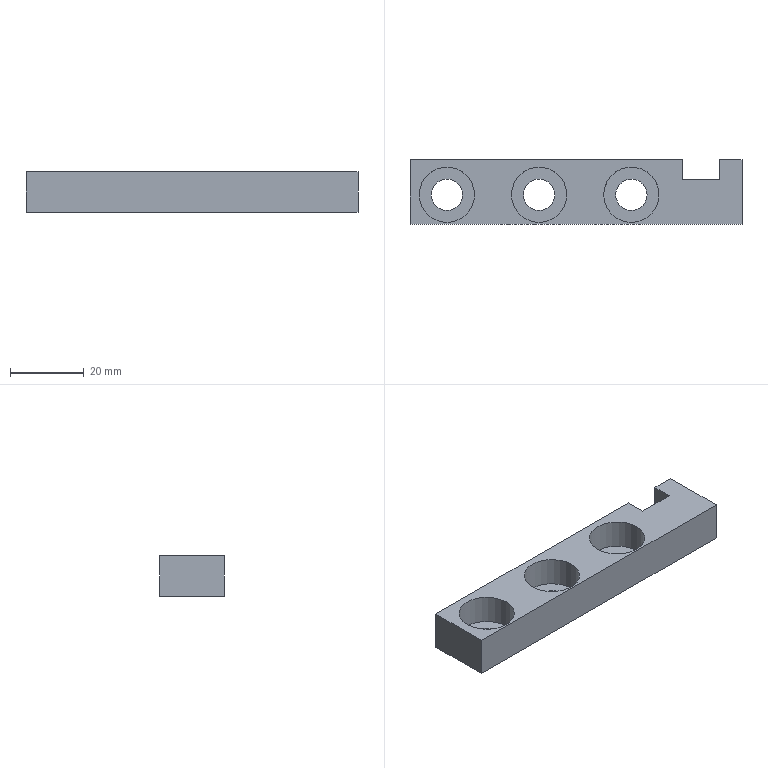Part | NX | features EXTRACT_STRING 6, EXTRUDE 6, EXTRACT_FACE 3, DATUM_CSYS 2, Instance Feature 2, BLOCK 1, Pattern Feature 1, RECT_SLOT 1, SKETCH 1 | 1 solid | 19 faces | box 90 x 17.5 x 11 mm | volume 11956 mm3 | plane 13 | cylinder 6 | commonest cylinder face diameters 8.5 x3 15 x3
STEP:
#1=CARTESIAN_POINT('',(90.,17.5,0.));
#2=VERTEX_POINT('',#1);
#3=CARTESIAN_POINT('',(84.,17.5,0.));
#4=VERTEX_POINT('',#3);
#5=CARTESIAN_POINT('',(45.,17.5,0.));
#6=DIRECTION('',(-1.,0.,0.));
#7=VECTOR('',#6,1000.);
#8=LINE('',#5,#7);
#9=EDGE_CURVE('',#2,#4,#8,.T.);
#10=ORIENTED_EDGE('',*,*,#9,.T.);
#11=CARTESIAN_POINT('',(84.,17.5,11.));
#12=VERTEX_POINT('',#11);
#13=CARTESIAN_POINT('',(84.,17.5,5.5));
#14=DIRECTION('',(0.,0.,1.));
#15=VECTOR('',#14,1000.);
#16=LINE('',#13,#15);
#17=EDGE_CURVE('',#4,#12,#16,.T.);
#18=ORIENTED_EDGE('',*,*,#17,.T.);
#19=CARTESIAN_POINT('',(90.,17.5,11.));
#20=VERTEX_POINT('',#19);
#21=CARTESIAN_POINT('',(45.,17.5,11.));
#22=DIRECTION('',(1.,0.,0.));
#23=VECTOR('',#22,1000.);
#24=LINE('',#21,#23);
#25=EDGE_CURVE('',#12,#20,#24,.T.);
#26=ORIENTED_EDGE('',*,*,#25,.T.);
#27=CARTESIAN_POINT('',(90.,17.5,0.));
#28=DIRECTION('',(0.,0.,1.));
#29=VECTOR('',#28,1000.);
#30=LINE('',#27,#29);
#31=EDGE_CURVE('',#2,#20,#30,.T.);
#32=ORIENTED_EDGE('',*,*,#31,.F.);
#33=EDGE_LOOP('',(#10,#18,#26,#32));
#34=FACE_BOUND('',#33,.T.);
#35=CARTESIAN_POINT('',(45.,17.5,0.));
#36=DIRECTION('',(0.,1.,0.));
#37=DIRECTION('',(0.,0.,1.));
#38=AXIS2_PLACEMENT_3D('',#35,#36,#37);
#39=PLANE('',#38);
#40=ADVANCED_FACE('',(#34),#39,.T.);
#41=CARTESIAN_POINT('',(17.5,8.,3.));
#42=VERTEX_POINT('',#41);
#43=CARTESIAN_POINT('',(10.,8.,3.));
#44=DIRECTION('',(0.,0.,-1.));
#45=DIRECTION('',(1.,0.,0.));
#46=AXIS2_PLACEMENT_3D('',#43,#44,#45);
#47=CIRCLE('',#46,7.5);
#48=EDGE_CURVE('',#42,#42,#47,.F.);
#49=ORIENTED_EDGE('',*,*,#48,.T.);
#50=EDGE_LOOP('',(#49));
#51=FACE_BOUND('',#50,.T.);
#52=CARTESIAN_POINT('',(5.75,8.,3.));
#53=VERTEX_POINT('',#52);
#54=CARTESIAN_POINT('',(10.,8.,3.));
#55=DIRECTION('',(0.,0.,-1.));
#56=DIRECTION('',(-1.,0.,0.));
#57=AXIS2_PLACEMENT_3D('',#54,#55,#56);
#58=CIRCLE('',#57,4.25);
#59=EDGE_CURVE('',#53,#53,#58,.F.);
#60=ORIENTED_EDGE('',*,*,#59,.F.);
#61=EDGE_LOOP('',(#60));
#62=FACE_BOUND('',#61,.T.);
#63=CARTESIAN_POINT('',(10.,8.,3.));
#64=DIRECTION('',(0.,0.,-1.));
#65=DIRECTION('',(-1.,0.,0.));
#66=AXIS2_PLACEMENT_3D('',#63,#64,#65);
#67=PLANE('',#66);
#68=ADVANCED_FACE('',(#51,#62),#67,.F.);
#69=CARTESIAN_POINT('',(84.,12.,11.));
#70=VERTEX_POINT('',#69);
#71=CARTESIAN_POINT('',(84.,8.75,11.));
#72=DIRECTION('',(0.,1.,0.));
#73=VECTOR('',#72,1000.);
#74=LINE('',#71,#73);
#75=EDGE_CURVE('',#70,#12,#74,.T.);
#76=ORIENTED_EDGE('',*,*,#75,.F.);
#77=CARTESIAN_POINT('',(73.8,12.,11.));
#78=VERTEX_POINT('',#77);
#79=CARTESIAN_POINT('',(45.,12.,11.));
#80=DIRECTION('',(1.,0.,0.));
#81=VECTOR('',#80,1000.);
#82=LINE('',#79,#81);
#83=EDGE_CURVE('',#78,#70,#82,.T.);
#84=ORIENTED_EDGE('',*,*,#83,.F.);
#85=CARTESIAN_POINT('',(73.8,17.5,11.));
#86=VERTEX_POINT('',#85);
#87=CARTESIAN_POINT('',(73.8,8.75,11.));
#88=DIRECTION('',(0.,-1.,0.));
#89=VECTOR('',#88,1000.);
#90=LINE('',#87,#89);
#91=EDGE_CURVE('',#86,#78,#90,.T.);
#92=ORIENTED_EDGE('',*,*,#91,.F.);
#93=CARTESIAN_POINT('',(0.,17.5,11.));
#94=VERTEX_POINT('',#93);
#95=CARTESIAN_POINT('',(45.,17.5,11.));
#96=DIRECTION('',(1.,0.,0.));
#97=VECTOR('',#96,1000.);
#98=LINE('',#95,#97);
#99=EDGE_CURVE('',#94,#86,#98,.T.);
#100=ORIENTED_EDGE('',*,*,#99,.F.);
#101=CARTESIAN_POINT('',(0.,0.,11.));
#102=VERTEX_POINT('',#101);
#103=CARTESIAN_POINT('',(0.,8.75,11.));
#104=DIRECTION('',(0.,1.,0.));
#105=VECTOR('',#104,1000.);
#106=LINE('',#103,#105);
#107=EDGE_CURVE('',#102,#94,#106,.T.);
#108=ORIENTED_EDGE('',*,*,#107,.F.);
#109=CARTESIAN_POINT('',(90.,0.,11.));
#110=VERTEX_POINT('',#109);
#111=CARTESIAN_POINT('',(45.,0.,11.));
#112=DIRECTION('',(-1.,0.,0.));
#113=VECTOR('',#112,1000.);
#114=LINE('',#111,#113);
#115=EDGE_CURVE('',#110,#102,#114,.T.);
#116=ORIENTED_EDGE('',*,*,#115,.F.);
#117=CARTESIAN_POINT('',(90.,8.75,11.));
#118=DIRECTION('',(0.,-1.,0.));
#119=VECTOR('',#118,1000.);
#120=LINE('',#117,#119);
#121=EDGE_CURVE('',#20,#110,#120,.T.);
#122=ORIENTED_EDGE('',*,*,#121,.F.);
#123=ORIENTED_EDGE('',*,*,#25,.F.);
#124=EDGE_LOOP('',(#76,#84,#92,#100,#108,#116,#122,#123));
#125=FACE_BOUND('',#124,.T.);
#126=CARTESIAN_POINT('',(42.5,8.,11.));
#127=VERTEX_POINT('',#126);
#128=CARTESIAN_POINT('',(35.,8.,11.));
#129=DIRECTION('',(0.,0.,-1.));
#130=DIRECTION('',(1.,0.,0.));
#131=AXIS2_PLACEMENT_3D('',#128,#129,#130);
#132=CIRCLE('',#131,7.5);
#133=EDGE_CURVE('',#127,#127,#132,.T.);
#134=ORIENTED_EDGE('',*,*,#133,.T.);
#135=EDGE_LOOP('',(#134));
#136=FACE_BOUND('',#135,.T.);
#137=CARTESIAN_POINT('',(67.5,8.,11.));
#138=VERTEX_POINT('',#137);
#139=CARTESIAN_POINT('',(60.,8.,11.));
#140=DIRECTION('',(0.,0.,-1.));
#141=DIRECTION('',(1.,0.,0.));
#142=AXIS2_PLACEMENT_3D('',#139,#140,#141);
#143=CIRCLE('',#142,7.5);
#144=EDGE_CURVE('',#138,#138,#143,.T.);
#145=ORIENTED_EDGE('',*,*,#144,.T.);
#146=EDGE_LOOP('',(#145));
#147=FACE_BOUND('',#146,.T.);
#148=CARTESIAN_POINT('',(17.5,8.,11.));
#149=VERTEX_POINT('',#148);
#150=CARTESIAN_POINT('',(10.,8.,11.));
#151=DIRECTION('',(0.,0.,-1.));
#152=DIRECTION('',(1.,0.,0.));
#153=AXIS2_PLACEMENT_3D('',#150,#151,#152);
#154=CIRCLE('',#153,7.5);
#155=EDGE_CURVE('',#149,#149,#154,.T.);
#156=ORIENTED_EDGE('',*,*,#155,.T.);
#157=EDGE_LOOP('',(#156));
#158=FACE_BOUND('',#157,.T.);
#159=CARTESIAN_POINT('',(45.,8.75,11.));
#160=DIRECTION('',(0.,0.,1.));
#161=DIRECTION('',(1.,0.,0.));
#162=AXIS2_PLACEMENT_3D('',#159,#160,#161);
#163=PLANE('',#162);
#164=ADVANCED_FACE('',(#125,#136,#147,#158),#163,.T.);
#165=CARTESIAN_POINT('',(42.5,8.,3.));
#166=VERTEX_POINT('',#165);
#167=CARTESIAN_POINT('',(35.,8.,3.));
#168=DIRECTION('',(0.,0.,-1.));
#169=DIRECTION('',(1.,0.,0.));
#170=AXIS2_PLACEMENT_3D('',#167,#168,#169);
#171=CIRCLE('',#170,7.5);
#172=EDGE_CURVE('',#166,#166,#171,.F.);
#173=ORIENTED_EDGE('',*,*,#172,.T.);
#174=EDGE_LOOP('',(#173));
#175=FACE_BOUND('',#174,.T.);
#176=CARTESIAN_POINT('',(30.75,8.,3.));
#177=VERTEX_POINT('',#176);
#178=CARTESIAN_POINT('',(35.,8.,3.));
#179=DIRECTION('',(0.,0.,-1.));
#180=DIRECTION('',(-1.,0.,0.));
#181=AXIS2_PLACEMENT_3D('',#178,#179,#180);
#182=CIRCLE('',#181,4.25);
#183=EDGE_CURVE('',#177,#177,#182,.F.);
#184=ORIENTED_EDGE('',*,*,#183,.F.);
#185=EDGE_LOOP('',(#184));
#186=FACE_BOUND('',#185,.T.);
#187=CARTESIAN_POINT('',(35.,8.,3.));
#188=DIRECTION('',(0.,0.,-1.));
#189=DIRECTION('',(-1.,0.,0.));
#190=AXIS2_PLACEMENT_3D('',#187,#188,#189);
#191=PLANE('',#190);
#192=ADVANCED_FACE('',(#175,#186),#191,.F.);
#193=CARTESIAN_POINT('',(67.5,8.,3.));
#194=VERTEX_POINT('',#193);
#195=CARTESIAN_POINT('',(60.,8.,3.));
#196=DIRECTION('',(0.,0.,-1.));
#197=DIRECTION('',(1.,0.,0.));
#198=AXIS2_PLACEMENT_3D('',#195,#196,#197);
#199=CIRCLE('',#198,7.5);
#200=EDGE_CURVE('',#194,#194,#199,.F.);
#201=ORIENTED_EDGE('',*,*,#200,.T.);
#202=EDGE_LOOP('',(#201));
#203=FACE_BOUND('',#202,.T.);
#204=CARTESIAN_POINT('',(55.75,8.,3.));
#205=VERTEX_POINT('',#204);
#206=CARTESIAN_POINT('',(60.,8.,3.));
#207=DIRECTION('',(0.,0.,-1.));
#208=DIRECTION('',(-1.,0.,0.));
#209=AXIS2_PLACEMENT_3D('',#206,#207,#208);
#210=CIRCLE('',#209,4.25);
#211=EDGE_CURVE('',#205,#205,#210,.F.);
#212=ORIENTED_EDGE('',*,*,#211,.F.);
#213=EDGE_LOOP('',(#212));
#214=FACE_BOUND('',#213,.T.);
#215=CARTESIAN_POINT('',(60.,8.,3.));
#216=DIRECTION('',(0.,0.,-1.));
#217=DIRECTION('',(-1.,0.,0.));
#218=AXIS2_PLACEMENT_3D('',#215,#216,#217);
#219=PLANE('',#218);
#220=ADVANCED_FACE('',(#203,#214),#219,.F.);
#221=CARTESIAN_POINT('',(90.,0.,0.));
#222=VERTEX_POINT('',#221);
#223=CARTESIAN_POINT('',(90.,0.,0.));
#224=DIRECTION('',(0.,0.,1.));
#225=VECTOR('',#224,1000.);
#226=LINE('',#223,#225);
#227=EDGE_CURVE('',#222,#110,#226,.T.);
#228=ORIENTED_EDGE('',*,*,#227,.T.);
#229=ORIENTED_EDGE('',*,*,#115,.T.);
#230=CARTESIAN_POINT('',(0.,0.,0.));
#231=VERTEX_POINT('',#230);
#232=CARTESIAN_POINT('',(0.,0.,0.));
#233=DIRECTION('',(0.,0.,1.));
#234=VECTOR('',#233,1000.);
#235=LINE('',#232,#234);
#236=EDGE_CURVE('',#231,#102,#235,.T.);
#237=ORIENTED_EDGE('',*,*,#236,.F.);
#238=CARTESIAN_POINT('',(45.,0.,0.));
#239=DIRECTION('',(1.,0.,0.));
#240=VECTOR('',#239,1000.);
#241=LINE('',#238,#240);
#242=EDGE_CURVE('',#231,#222,#241,.T.);
#243=ORIENTED_EDGE('',*,*,#242,.T.);
#244=EDGE_LOOP('',(#228,#229,#237,#243));
#245=FACE_BOUND('',#244,.T.);
#246=CARTESIAN_POINT('',(45.,0.,0.));
#247=DIRECTION('',(0.,-1.,0.));
#248=DIRECTION('',(0.,0.,-1.));
#249=AXIS2_PLACEMENT_3D('',#246,#247,#248);
#250=PLANE('',#249);
#251=ADVANCED_FACE('',(#245),#250,.T.);
#252=ORIENTED_EDGE('',*,*,#236,.T.);
#253=ORIENTED_EDGE('',*,*,#107,.T.);
#254=CARTESIAN_POINT('',(0.,17.5,0.));
#255=VERTEX_POINT('',#254);
#256=CARTESIAN_POINT('',(0.,17.5,0.));
#257=DIRECTION('',(0.,0.,1.));
#258=VECTOR('',#257,1000.);
#259=LINE('',#256,#258);
#260=EDGE_CURVE('',#255,#94,#259,.T.);
#261=ORIENTED_EDGE('',*,*,#260,.F.);
#262=CARTESIAN_POINT('',(0.,8.75,0.));
#263=DIRECTION('',(0.,-1.,0.));
#264=VECTOR('',#263,1000.);
#265=LINE('',#262,#264);
#266=EDGE_CURVE('',#255,#231,#265,.T.);
#267=ORIENTED_EDGE('',*,*,#266,.T.);
#268=EDGE_LOOP('',(#252,#253,#261,#267));
#269=FACE_BOUND('',#268,.T.);
#270=CARTESIAN_POINT('',(0.,8.75,0.));
#271=DIRECTION('',(-1.,0.,0.));
#272=DIRECTION('',(0.,0.,1.));
#273=AXIS2_PLACEMENT_3D('',#270,#271,#272);
#274=PLANE('',#273);
#275=ADVANCED_FACE('',(#269),#274,.T.);
#276=CARTESIAN_POINT('',(73.8,17.5,0.));
#277=VERTEX_POINT('',#276);
#278=CARTESIAN_POINT('',(73.8,17.5,5.5));
#279=DIRECTION('',(0.,0.,1.));
#280=VECTOR('',#279,1000.);
#281=LINE('',#278,#280);
#282=EDGE_CURVE('',#277,#86,#281,.T.);
#283=ORIENTED_EDGE('',*,*,#282,.F.);
#284=CARTESIAN_POINT('',(45.,17.5,0.));
#285=DIRECTION('',(-1.,0.,0.));
#286=VECTOR('',#285,1000.);
#287=LINE('',#284,#286);
#288=EDGE_CURVE('',#277,#255,#287,.T.);
#289=ORIENTED_EDGE('',*,*,#288,.T.);
#290=ORIENTED_EDGE('',*,*,#260,.T.);
#291=ORIENTED_EDGE('',*,*,#99,.T.);
#292=EDGE_LOOP('',(#283,#289,#290,#291));
#293=FACE_BOUND('',#292,.T.);
#294=CARTESIAN_POINT('',(45.,17.5,0.));
#295=DIRECTION('',(0.,1.,0.));
#296=DIRECTION('',(0.,0.,1.));
#297=AXIS2_PLACEMENT_3D('',#294,#295,#296);
#298=PLANE('',#297);
#299=ADVANCED_FACE('',(#293),#298,.T.);
#300=CARTESIAN_POINT('',(84.,12.,0.));
#301=VERTEX_POINT('',#300);
#302=CARTESIAN_POINT('',(84.,8.75,0.));
#303=DIRECTION('',(0.,-1.,0.));
#304=VECTOR('',#303,1000.);
#305=LINE('',#302,#304);
#306=EDGE_CURVE('',#4,#301,#305,.T.);
#307=ORIENTED_EDGE('',*,*,#306,.F.);
#308=ORIENTED_EDGE('',*,*,#9,.F.);
#309=CARTESIAN_POINT('',(90.,8.75,0.));
#310=DIRECTION('',(0.,1.,0.));
#311=VECTOR('',#310,1000.);
#312=LINE('',#309,#311);
#313=EDGE_CURVE('',#222,#2,#312,.T.);
#314=ORIENTED_EDGE('',*,*,#313,.F.);
#315=ORIENTED_EDGE('',*,*,#242,.F.);
#316=ORIENTED_EDGE('',*,*,#266,.F.);
#317=ORIENTED_EDGE('',*,*,#288,.F.);
#318=CARTESIAN_POINT('',(73.8,12.,0.));
#319=VERTEX_POINT('',#318);
#320=CARTESIAN_POINT('',(73.8,8.75,0.));
#321=DIRECTION('',(0.,1.,0.));
#322=VECTOR('',#321,1000.);
#323=LINE('',#320,#322);
#324=EDGE_CURVE('',#319,#277,#323,.T.);
#325=ORIENTED_EDGE('',*,*,#324,.F.);
#326=CARTESIAN_POINT('',(45.,12.,0.));
#327=DIRECTION('',(-1.,0.,0.));
#328=VECTOR('',#327,1000.);
#329=LINE('',#326,#328);
#330=EDGE_CURVE('',#301,#319,#329,.T.);
#331=ORIENTED_EDGE('',*,*,#330,.F.);
#332=EDGE_LOOP('',(#307,#308,#314,#315,#316,#317,#325,#331));
#333=FACE_BOUND('',#332,.T.);
#334=CARTESIAN_POINT('',(5.75,8.,0.));
#335=VERTEX_POINT('',#334);
#336=CARTESIAN_POINT('',(10.,8.,0.));
#337=DIRECTION('',(0.,0.,-1.));
#338=DIRECTION('',(-1.,0.,0.));
#339=AXIS2_PLACEMENT_3D('',#336,#337,#338);
#340=CIRCLE('',#339,4.25);
#341=EDGE_CURVE('',#335,#335,#340,.T.);
#342=ORIENTED_EDGE('',*,*,#341,.F.);
#343=EDGE_LOOP('',(#342));
#344=FACE_BOUND('',#343,.T.);
#345=CARTESIAN_POINT('',(30.75,8.,0.));
#346=VERTEX_POINT('',#345);
#347=CARTESIAN_POINT('',(35.,8.,0.));
#348=DIRECTION('',(0.,0.,-1.));
#349=DIRECTION('',(-1.,0.,0.));
#350=AXIS2_PLACEMENT_3D('',#347,#348,#349);
#351=CIRCLE('',#350,4.25);
#352=EDGE_CURVE('',#346,#346,#351,.T.);
#353=ORIENTED_EDGE('',*,*,#352,.F.);
#354=EDGE_LOOP('',(#353));
#355=FACE_BOUND('',#354,.T.);
#356=CARTESIAN_POINT('',(55.75,8.,0.));
#357=VERTEX_POINT('',#356);
#358=CARTESIAN_POINT('',(60.,8.,0.));
#359=DIRECTION('',(0.,0.,-1.));
#360=DIRECTION('',(-1.,0.,0.));
#361=AXIS2_PLACEMENT_3D('',#358,#359,#360);
#362=CIRCLE('',#361,4.25);
#363=EDGE_CURVE('',#357,#357,#362,.T.);
#364=ORIENTED_EDGE('',*,*,#363,.F.);
#365=EDGE_LOOP('',(#364));
#366=FACE_BOUND('',#365,.T.);
#367=CARTESIAN_POINT('',(45.,8.75,0.));
#368=DIRECTION('',(0.,0.,-1.));
#369=DIRECTION('',(-1.,0.,0.));
#370=AXIS2_PLACEMENT_3D('',#367,#368,#369);
#371=PLANE('',#370);
#372=ADVANCED_FACE('',(#333,#344,#355,#366),#371,.T.);
#373=ORIENTED_EDGE('',*,*,#313,.T.);
#374=ORIENTED_EDGE('',*,*,#31,.T.);
#375=ORIENTED_EDGE('',*,*,#121,.T.);
#376=ORIENTED_EDGE('',*,*,#227,.F.);
#377=EDGE_LOOP('',(#373,#374,#375,#376));
#378=FACE_BOUND('',#377,.T.);
#379=CARTESIAN_POINT('',(90.,8.75,0.));
#380=DIRECTION('',(1.,0.,0.));
#381=DIRECTION('',(0.,0.,-1.));
#382=AXIS2_PLACEMENT_3D('',#379,#380,#381);
#383=PLANE('',#382);
#384=ADVANCED_FACE('',(#378),#383,.T.);
#385=ORIENTED_EDGE('',*,*,#200,.F.);
#386=EDGE_LOOP('',(#385));
#387=FACE_BOUND('',#386,.T.);
#388=ORIENTED_EDGE('',*,*,#144,.F.);
#389=EDGE_LOOP('',(#388));
#390=FACE_BOUND('',#389,.T.);
#391=CARTESIAN_POINT('',(60.,8.,3.));
#392=DIRECTION('',(0.,0.,1.));
#393=DIRECTION('',(1.,0.,0.));
#394=AXIS2_PLACEMENT_3D('',#391,#392,#393);
#395=CYLINDRICAL_SURFACE('',#394,7.5);
#396=ADVANCED_FACE('',(#387,#390),#395,.F.);
#397=ORIENTED_EDGE('',*,*,#363,.T.);
#398=EDGE_LOOP('',(#397));
#399=FACE_BOUND('',#398,.T.);
#400=ORIENTED_EDGE('',*,*,#211,.T.);
#401=EDGE_LOOP('',(#400));
#402=FACE_BOUND('',#401,.T.);
#403=CARTESIAN_POINT('',(60.,8.,-97.9));
#404=DIRECTION('',(0.,0.,1.));
#405=DIRECTION('',(1.,0.,0.));
#406=AXIS2_PLACEMENT_3D('',#403,#404,#405);
#407=CYLINDRICAL_SURFACE('',#406,4.25);
#408=ADVANCED_FACE('',(#399,#402),#407,.F.);
#409=ORIENTED_EDGE('',*,*,#172,.F.);
#410=EDGE_LOOP('',(#409));
#411=FACE_BOUND('',#410,.T.);
#412=ORIENTED_EDGE('',*,*,#133,.F.);
#413=EDGE_LOOP('',(#412));
#414=FACE_BOUND('',#413,.T.);
#415=CARTESIAN_POINT('',(35.,8.,3.));
#416=DIRECTION('',(0.,0.,1.));
#417=DIRECTION('',(1.,0.,0.));
#418=AXIS2_PLACEMENT_3D('',#415,#416,#417);
#419=CYLINDRICAL_SURFACE('',#418,7.5);
#420=ADVANCED_FACE('',(#411,#414),#419,.F.);
#421=ORIENTED_EDGE('',*,*,#352,.T.);
#422=EDGE_LOOP('',(#421));
#423=FACE_BOUND('',#422,.T.);
#424=ORIENTED_EDGE('',*,*,#183,.T.);
#425=EDGE_LOOP('',(#424));
#426=FACE_BOUND('',#425,.T.);
#427=CARTESIAN_POINT('',(35.,8.,-97.9));
#428=DIRECTION('',(0.,0.,1.));
#429=DIRECTION('',(1.,0.,0.));
#430=AXIS2_PLACEMENT_3D('',#427,#428,#429);
#431=CYLINDRICAL_SURFACE('',#430,4.25);
#432=ADVANCED_FACE('',(#423,#426),#431,.F.);
#433=ORIENTED_EDGE('',*,*,#48,.F.);
#434=EDGE_LOOP('',(#433));
#435=FACE_BOUND('',#434,.T.);
#436=ORIENTED_EDGE('',*,*,#155,.F.);
#437=EDGE_LOOP('',(#436));
#438=FACE_BOUND('',#437,.T.);
#439=CARTESIAN_POINT('',(10.,8.,3.));
#440=DIRECTION('',(0.,0.,1.));
#441=DIRECTION('',(1.,0.,0.));
#442=AXIS2_PLACEMENT_3D('',#439,#440,#441);
#443=CYLINDRICAL_SURFACE('',#442,7.5);
#444=ADVANCED_FACE('',(#435,#438),#443,.F.);
#445=ORIENTED_EDGE('',*,*,#341,.T.);
#446=EDGE_LOOP('',(#445));
#447=FACE_BOUND('',#446,.T.);
#448=ORIENTED_EDGE('',*,*,#59,.T.);
#449=EDGE_LOOP('',(#448));
#450=FACE_BOUND('',#449,.T.);
#451=CARTESIAN_POINT('',(10.,8.,-97.9));
#452=DIRECTION('',(0.,0.,1.));
#453=DIRECTION('',(1.,0.,0.));
#454=AXIS2_PLACEMENT_3D('',#451,#452,#453);
#455=CYLINDRICAL_SURFACE('',#454,4.25);
#456=ADVANCED_FACE('',(#447,#450),#455,.F.);
#457=ORIENTED_EDGE('',*,*,#306,.T.);
#458=CARTESIAN_POINT('',(84.,12.,-25.848));
#459=DIRECTION('',(0.,0.,1.));
#460=VECTOR('',#459,1000.);
#461=LINE('',#458,#460);
#462=EDGE_CURVE('',#70,#301,#461,.F.);
#463=ORIENTED_EDGE('',*,*,#462,.F.);
#464=ORIENTED_EDGE('',*,*,#75,.T.);
#465=ORIENTED_EDGE('',*,*,#17,.F.);
#466=EDGE_LOOP('',(#457,#463,#464,#465));
#467=FACE_BOUND('',#466,.T.);
#468=CARTESIAN_POINT('',(84.,17.5,5.5));
#469=DIRECTION('',(1.,0.,0.));
#470=DIRECTION('',(0.,0.,-1.));
#471=AXIS2_PLACEMENT_3D('',#468,#469,#470);
#472=PLANE('',#471);
#473=ADVANCED_FACE('',(#467),#472,.F.);
#474=ORIENTED_EDGE('',*,*,#330,.T.);
#475=CARTESIAN_POINT('',(73.8,12.,-25.848));
#476=DIRECTION('',(0.,0.,1.));
#477=VECTOR('',#476,1000.);
#478=LINE('',#475,#477);
#479=EDGE_CURVE('',#78,#319,#478,.F.);
#480=ORIENTED_EDGE('',*,*,#479,.F.);
#481=ORIENTED_EDGE('',*,*,#83,.T.);
#482=ORIENTED_EDGE('',*,*,#462,.T.);
#483=EDGE_LOOP('',(#474,#480,#481,#482));
#484=FACE_BOUND('',#483,.T.);
#485=CARTESIAN_POINT('',(78.9,12.,5.5));
#486=DIRECTION('',(0.,-1.,0.));
#487=DIRECTION('',(0.,0.,-1.));
#488=AXIS2_PLACEMENT_3D('',#485,#486,#487);
#489=PLANE('',#488);
#490=ADVANCED_FACE('',(#484),#489,.F.);
#491=ORIENTED_EDGE('',*,*,#324,.T.);
#492=ORIENTED_EDGE('',*,*,#282,.T.);
#493=ORIENTED_EDGE('',*,*,#91,.T.);
#494=ORIENTED_EDGE('',*,*,#479,.T.);
#495=EDGE_LOOP('',(#491,#492,#493,#494));
#496=FACE_BOUND('',#495,.T.);
#497=CARTESIAN_POINT('',(73.8,17.5,5.5));
#498=DIRECTION('',(-1.,0.,0.));
#499=DIRECTION('',(0.,0.,1.));
#500=AXIS2_PLACEMENT_3D('',#497,#498,#499);
#501=PLANE('',#500);
#502=ADVANCED_FACE('',(#496),#501,.F.);
#503=CLOSED_SHELL('',(#40,#68,#164,#192,#220,#251,#275,#299,#372,#384,#396,#408,#420,#432,#444,#456,#473,#490,#502));
#504=MANIFOLD_SOLID_BREP('',#503);
#505=(LENGTH_UNIT()NAMED_UNIT(*)SI_UNIT(.MILLI.,.METRE.));
#506=UNCERTAINTY_MEASURE_WITH_UNIT(LENGTH_MEASURE(0.00001),#505,'','');
#507=(NAMED_UNIT(*)PLANE_ANGLE_UNIT()SI_UNIT($,.RADIAN.));
#508=(NAMED_UNIT(*)SI_UNIT($,.STERADIAN.)SOLID_ANGLE_UNIT());
#509=(GEOMETRIC_REPRESENTATION_CONTEXT(3)GLOBAL_UNCERTAINTY_ASSIGNED_CONTEXT((#506))GLOBAL_UNIT_ASSIGNED_CONTEXT((#505,#507,#508))REPRESENTATION_CONTEXT('',''));
#510=ADVANCED_BREP_SHAPE_REPRESENTATION('',(#504),#509);